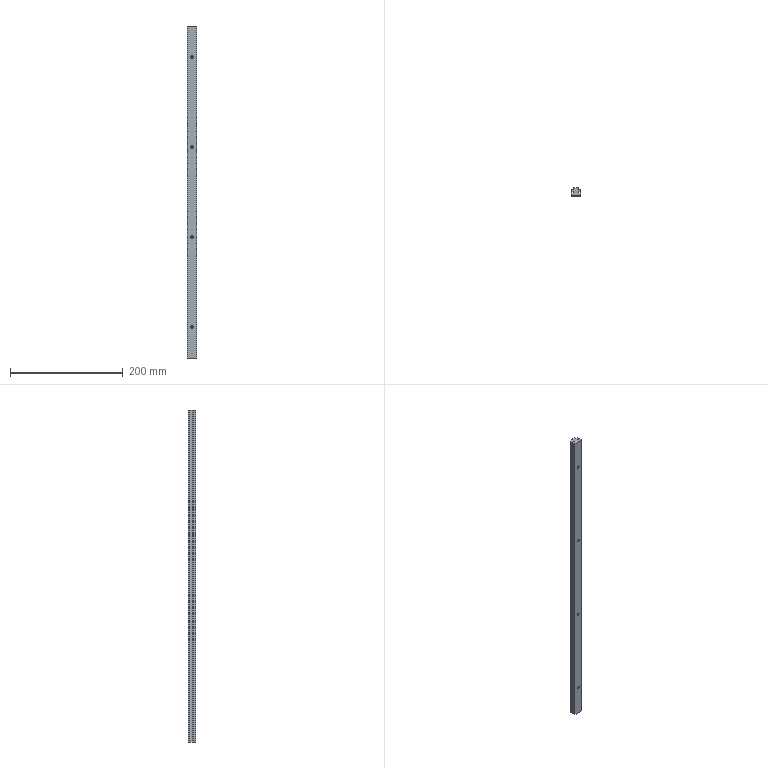Part | STEP file | 0228_Z_LGTS40-590-K4-P1601 | 1 solid | 36 faces | box 17 x 14 x 590 mm | volume 119990 mm3 | plane 20 | cylinder 8 | cone 8 | commonest cylinder face diameters 4.2 x8